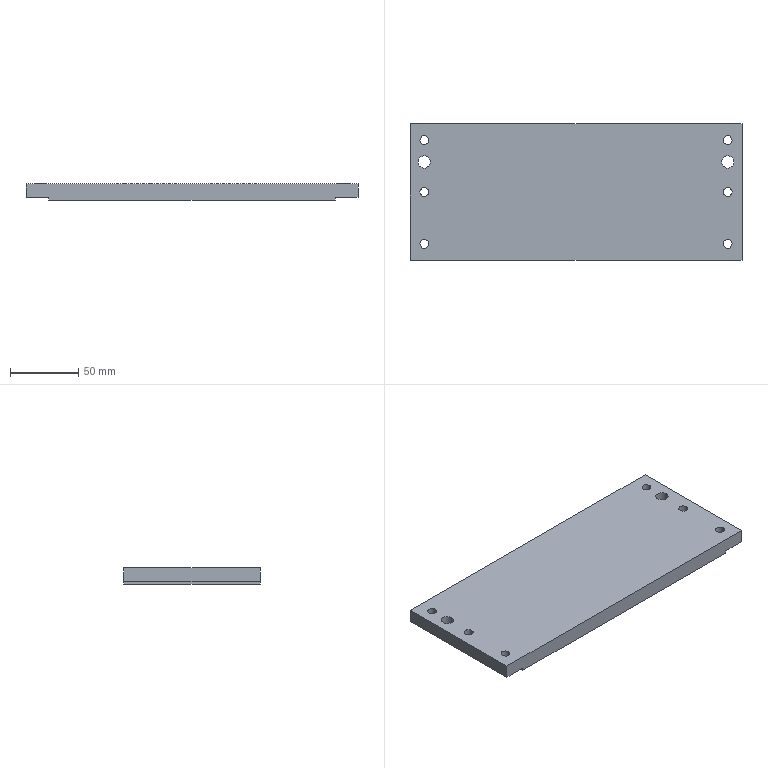Part | STEP file | 0228_212_Plate | 1 solid | 26 faces | box 243 x 100 x 12 mm | volume 281737 mm3 | cylinder 16 | plane 10 | commonest cylinder face diameters 6.5 x12 9 x4